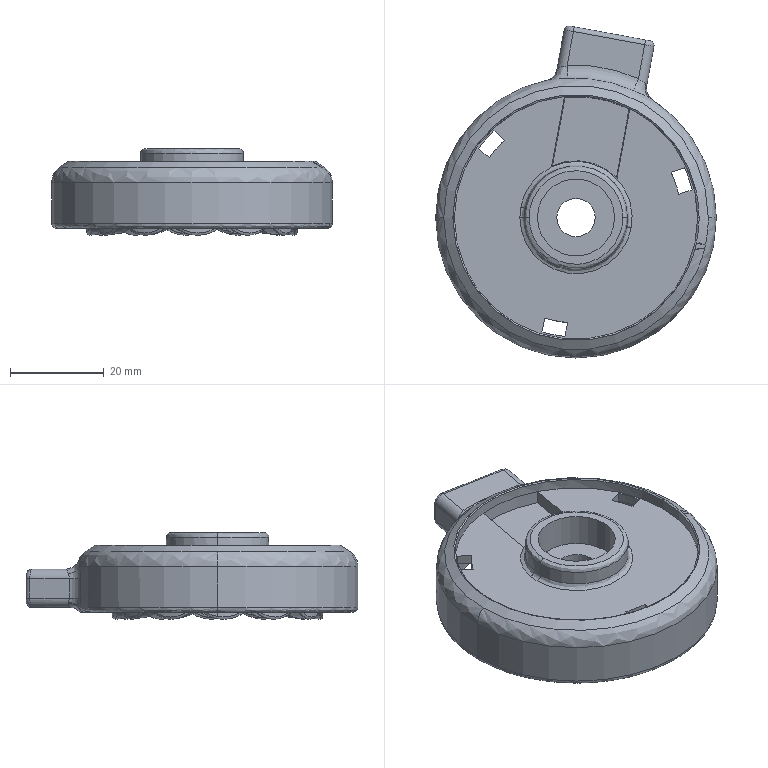Part | SolidWorks | features BaseBody 1 | 1 solid | 204 faces | box 60 x 70.94 x 18.527 mm | volume 21713 mm3 | spline 107 | cylinder 49 | plane 29 | torus 15 | cone 2 | sphere 2 | commonest cylinder face diameters 2 x11 4 x8 22 x5 6 x3 51 x3 60 x3